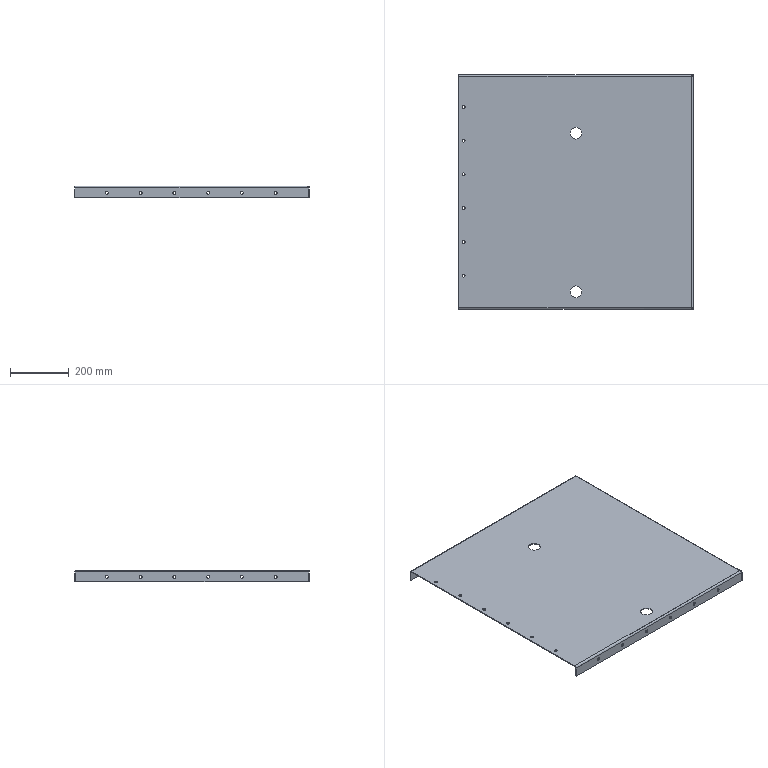Part | SolidWorks | features ICE 4, CornerFeat 1, EdgeFlange 1, FlatPattern 1, SMBaseFlange 1, SheetMetal 1 | 1 solid | 82 faces | box 800 x 800 x 40 mm | volume 2158563 mm3 | cylinder 58 | plane 20 | spline 4 | commonest cylinder face diameters 10 x48 40 x4 6 x3 12 x3